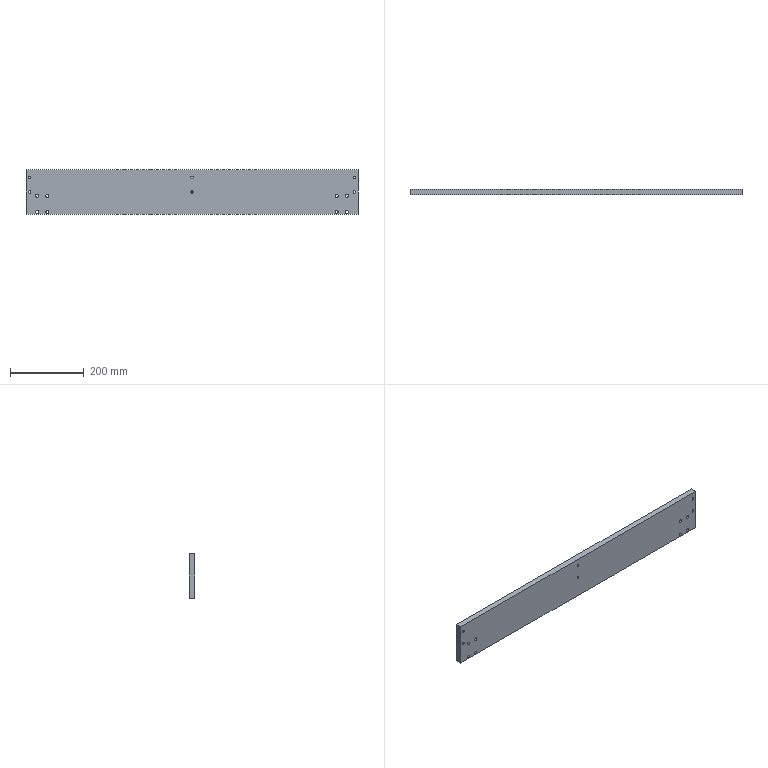Part | SolidWorks | features HoleWzd 2, Extrusion 1, LPattern 1, MirrorPattern 1 | 1 solid | 52 faces | box 900 x 16 x 120 mm | volume 1714971 mm3 | cylinder 40 | plane 12 | commonest cylinder face diameters 8.5 x16 6.6 x12 11 x12